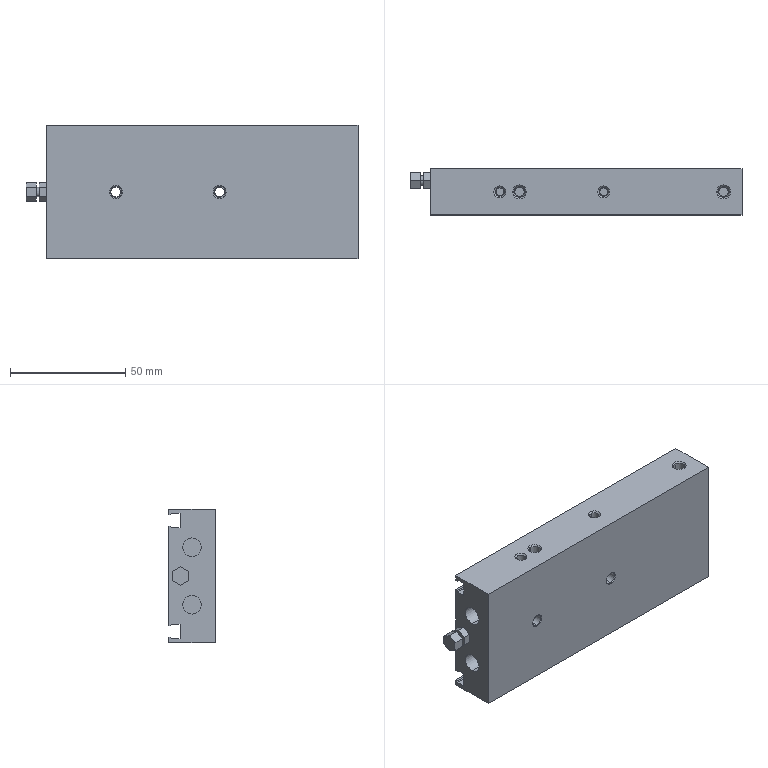Part | NX | 1 solid | 163 faces | box 144 x 20 x 58 mm | volume 134254 mm3 | cylinder 62 | plane 53 | cone 48 | commonest cylinder face diameters 4 x18 5 x12 3.4 x8 4.5 x8 8 x8 4.3 x4